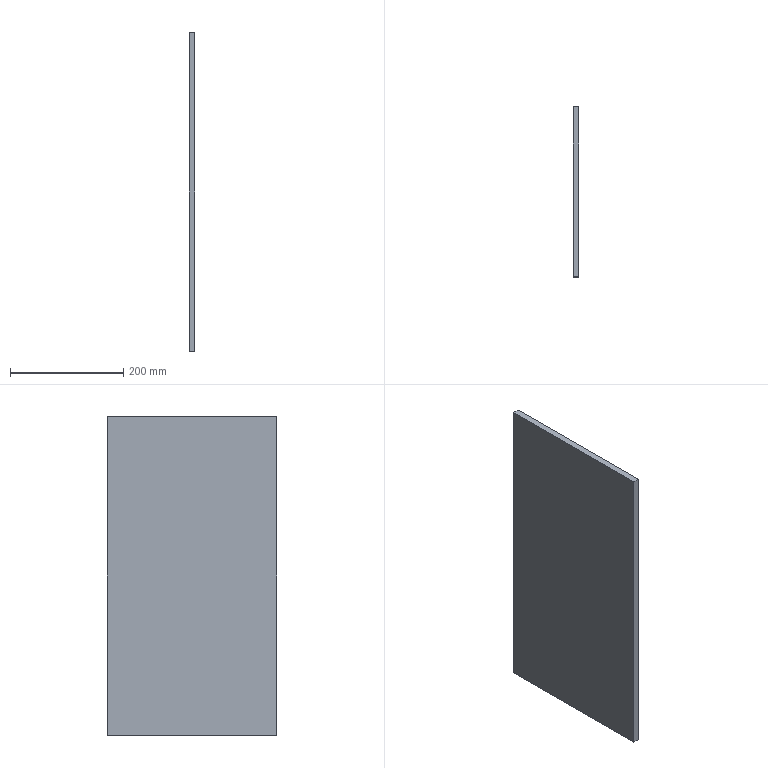Part | SolidWorks | features Extrusion 1 | 1 solid | 6 faces | box 10.5 x 300 x 563.2 mm | volume 1774080 mm3 | plane 6
STEP:
#1=CARTESIAN_POINT('',(0.,300.,0.));
#2=VERTEX_POINT('',#1);
#3=CARTESIAN_POINT('',(0.,0.,0.));
#4=VERTEX_POINT('',#3);
#5=CARTESIAN_POINT('',(0.,0.,0.));
#6=DIRECTION('',(0.,-1.,0.));
#7=VECTOR('',#6,1000.);
#8=LINE('',#5,#7);
#9=EDGE_CURVE('',#2,#4,#8,.T.);
#10=ORIENTED_EDGE('',*,*,#9,.T.);
#11=CARTESIAN_POINT('',(10.5,0.,0.));
#12=VERTEX_POINT('',#11);
#13=CARTESIAN_POINT('',(10.5,0.,0.));
#14=DIRECTION('',(-1.,0.,0.));
#15=VECTOR('',#14,1000.);
#16=LINE('',#13,#15);
#17=EDGE_CURVE('',#12,#4,#16,.T.);
#18=ORIENTED_EDGE('',*,*,#17,.F.);
#19=CARTESIAN_POINT('',(10.5,300.,0.));
#20=VERTEX_POINT('',#19);
#21=CARTESIAN_POINT('',(10.5,0.,0.));
#22=DIRECTION('',(0.,-1.,0.));
#23=VECTOR('',#22,1000.);
#24=LINE('',#21,#23);
#25=EDGE_CURVE('',#20,#12,#24,.T.);
#26=ORIENTED_EDGE('',*,*,#25,.F.);
#27=CARTESIAN_POINT('',(10.5,300.,0.));
#28=DIRECTION('',(-1.,0.,0.));
#29=VECTOR('',#28,1000.);
#30=LINE('',#27,#29);
#31=EDGE_CURVE('',#20,#2,#30,.T.);
#32=ORIENTED_EDGE('',*,*,#31,.T.);
#33=EDGE_LOOP('',(#10,#18,#26,#32));
#34=FACE_OUTER_BOUND('',#33,.T.);
#35=CARTESIAN_POINT('',(10.5,0.,0.));
#36=DIRECTION('',(0.,0.,-1.));
#37=DIRECTION('',(-1.,0.,0.));
#38=AXIS2_PLACEMENT_3D('',#35,#36,#37);
#39=PLANE('',#38);
#40=ADVANCED_FACE('',(#34),#39,.F.);
#41=CARTESIAN_POINT('',(0.,0.,-563.2));
#42=VERTEX_POINT('',#41);
#43=CARTESIAN_POINT('',(0.,0.,0.));
#44=DIRECTION('',(0.,0.,-1.));
#45=VECTOR('',#44,1000.);
#46=LINE('',#43,#45);
#47=EDGE_CURVE('',#4,#42,#46,.T.);
#48=ORIENTED_EDGE('',*,*,#47,.T.);
#49=CARTESIAN_POINT('',(10.5,0.,-563.2));
#50=VERTEX_POINT('',#49);
#51=CARTESIAN_POINT('',(10.5,0.,-563.2));
#52=DIRECTION('',(-1.,0.,0.));
#53=VECTOR('',#52,1000.);
#54=LINE('',#51,#53);
#55=EDGE_CURVE('',#50,#42,#54,.T.);
#56=ORIENTED_EDGE('',*,*,#55,.F.);
#57=CARTESIAN_POINT('',(10.5,0.,0.));
#58=DIRECTION('',(0.,0.,-1.));
#59=VECTOR('',#58,1000.);
#60=LINE('',#57,#59);
#61=EDGE_CURVE('',#12,#50,#60,.T.);
#62=ORIENTED_EDGE('',*,*,#61,.F.);
#63=ORIENTED_EDGE('',*,*,#17,.T.);
#64=EDGE_LOOP('',(#48,#56,#62,#63));
#65=FACE_OUTER_BOUND('',#64,.T.);
#66=CARTESIAN_POINT('',(10.5,0.,0.));
#67=DIRECTION('',(0.,1.,0.));
#68=DIRECTION('',(0.,0.,1.));
#69=AXIS2_PLACEMENT_3D('',#66,#67,#68);
#70=PLANE('',#69);
#71=ADVANCED_FACE('',(#65),#70,.F.);
#72=CARTESIAN_POINT('',(0.,300.,-563.2));
#73=VERTEX_POINT('',#72);
#74=CARTESIAN_POINT('',(0.,0.,-563.2));
#75=DIRECTION('',(0.,1.,0.));
#76=VECTOR('',#75,1000.);
#77=LINE('',#74,#76);
#78=EDGE_CURVE('',#42,#73,#77,.T.);
#79=ORIENTED_EDGE('',*,*,#78,.T.);
#80=CARTESIAN_POINT('',(10.5,300.,-563.2));
#81=VERTEX_POINT('',#80);
#82=CARTESIAN_POINT('',(10.5,300.,-563.2));
#83=DIRECTION('',(-1.,0.,0.));
#84=VECTOR('',#83,1000.);
#85=LINE('',#82,#84);
#86=EDGE_CURVE('',#81,#73,#85,.T.);
#87=ORIENTED_EDGE('',*,*,#86,.F.);
#88=CARTESIAN_POINT('',(10.5,0.,-563.2));
#89=DIRECTION('',(0.,1.,0.));
#90=VECTOR('',#89,1000.);
#91=LINE('',#88,#90);
#92=EDGE_CURVE('',#50,#81,#91,.T.);
#93=ORIENTED_EDGE('',*,*,#92,.F.);
#94=ORIENTED_EDGE('',*,*,#55,.T.);
#95=EDGE_LOOP('',(#79,#87,#93,#94));
#96=FACE_OUTER_BOUND('',#95,.T.);
#97=CARTESIAN_POINT('',(10.5,0.,-563.2));
#98=DIRECTION('',(0.,0.,1.));
#99=DIRECTION('',(1.,0.,0.));
#100=AXIS2_PLACEMENT_3D('',#97,#98,#99);
#101=PLANE('',#100);
#102=ADVANCED_FACE('',(#96),#101,.F.);
#103=CARTESIAN_POINT('',(0.,300.,0.));
#104=DIRECTION('',(0.,0.,1.));
#105=VECTOR('',#104,1000.);
#106=LINE('',#103,#105);
#107=EDGE_CURVE('',#73,#2,#106,.T.);
#108=ORIENTED_EDGE('',*,*,#107,.T.);
#109=ORIENTED_EDGE('',*,*,#31,.F.);
#110=CARTESIAN_POINT('',(10.5,300.,0.));
#111=DIRECTION('',(0.,0.,1.));
#112=VECTOR('',#111,1000.);
#113=LINE('',#110,#112);
#114=EDGE_CURVE('',#81,#20,#113,.T.);
#115=ORIENTED_EDGE('',*,*,#114,.F.);
#116=ORIENTED_EDGE('',*,*,#86,.T.);
#117=EDGE_LOOP('',(#108,#109,#115,#116));
#118=FACE_OUTER_BOUND('',#117,.T.);
#119=CARTESIAN_POINT('',(10.5,300.,0.));
#120=DIRECTION('',(0.,-1.,0.));
#121=DIRECTION('',(0.,0.,-1.));
#122=AXIS2_PLACEMENT_3D('',#119,#120,#121);
#123=PLANE('',#122);
#124=ADVANCED_FACE('',(#118),#123,.F.);
#125=ORIENTED_EDGE('',*,*,#25,.T.);
#126=ORIENTED_EDGE('',*,*,#61,.T.);
#127=ORIENTED_EDGE('',*,*,#92,.T.);
#128=ORIENTED_EDGE('',*,*,#114,.T.);
#129=EDGE_LOOP('',(#125,#126,#127,#128));
#130=FACE_OUTER_BOUND('',#129,.T.);
#131=CARTESIAN_POINT('',(10.5,0.,0.));
#132=DIRECTION('',(-1.,0.,0.));
#133=DIRECTION('',(0.,0.,1.));
#134=AXIS2_PLACEMENT_3D('',#131,#132,#133);
#135=PLANE('',#134);
#136=ADVANCED_FACE('',(#130),#135,.F.);
#137=ORIENTED_EDGE('',*,*,#9,.F.);
#138=ORIENTED_EDGE('',*,*,#107,.F.);
#139=ORIENTED_EDGE('',*,*,#78,.F.);
#140=ORIENTED_EDGE('',*,*,#47,.F.);
#141=EDGE_LOOP('',(#137,#138,#139,#140));
#142=FACE_OUTER_BOUND('',#141,.T.);
#143=CARTESIAN_POINT('',(0.,0.,0.));
#144=DIRECTION('',(-1.,0.,0.));
#145=DIRECTION('',(0.,0.,1.));
#146=AXIS2_PLACEMENT_3D('',#143,#144,#145);
#147=PLANE('',#146);
#148=ADVANCED_FACE('',(#142),#147,.T.);
#149=CLOSED_SHELL('',(#40,#71,#102,#124,#136,#148));
#150=MANIFOLD_SOLID_BREP('',#149);
#151=CARTESIAN_POINT('',(0.,0.,0.));
#152=DIRECTION('',(0.,0.,1.));
#153=DIRECTION('',(1.,0.,0.));
#154=AXIS2_PLACEMENT_3D('',#151,#152,#153);
#155=(LENGTH_UNIT()NAMED_UNIT(*)SI_UNIT(.MILLI.,.METRE.));
#156=UNCERTAINTY_MEASURE_WITH_UNIT(LENGTH_MEASURE(0.00001),#155,'','');
#157=(NAMED_UNIT(*)PLANE_ANGLE_UNIT()SI_UNIT($,.RADIAN.));
#158=(NAMED_UNIT(*)SI_UNIT($,.STERADIAN.)SOLID_ANGLE_UNIT());
#159=(GEOMETRIC_REPRESENTATION_CONTEXT(3)GLOBAL_UNCERTAINTY_ASSIGNED_CONTEXT((#156))GLOBAL_UNIT_ASSIGNED_CONTEXT((#155,#157,#158))REPRESENTATION_CONTEXT('',''));
#160=ADVANCED_BREP_SHAPE_REPRESENTATION('',(#150,#154),#159);